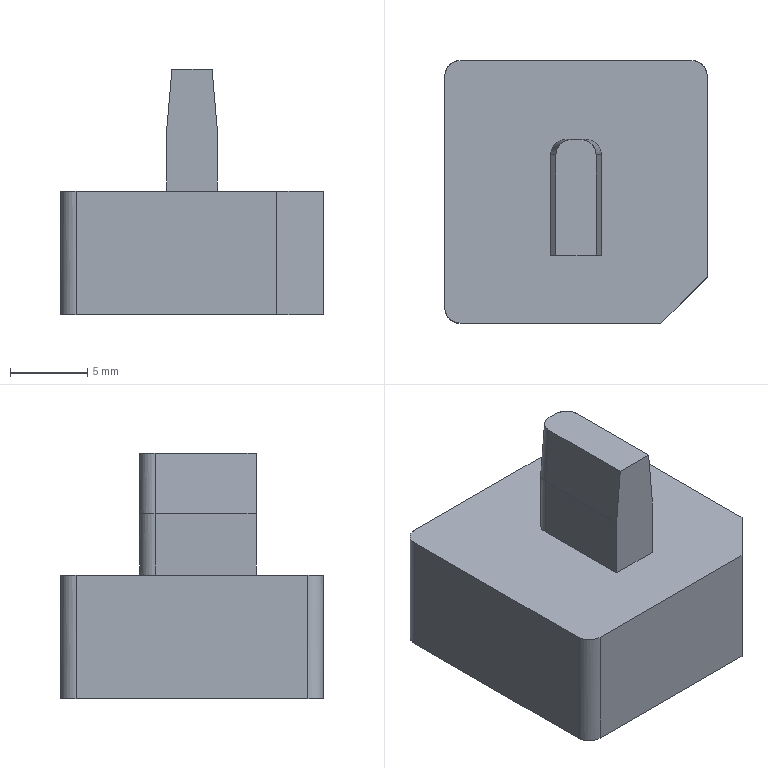NC program | PowerMill | posted with a generic post | part box 17 x 17 x 15.883 mm
Lines 3250 to 4049 of 22972:
N3347 M6
N3348 S18000 M03
N3349 G00 G90 X0.0 Y0.0
N3350 G43 Z10.804 H14
N3351
N3352 G05 P10000 R8
N3353 X2.8538 Y-6.1498
N3354 Z0.7597
N3355 G01 Z-0.4403 F1200.0
N3356 X2.8235 Y-6.0851 F2000.0
N3357 X2.7862 Y-6.0242
N3358 X2.7423 Y-5.9678
N3359 X2.6924 Y-5.9166
N3360 X2.6371 Y-5.8714
N3361 X2.5772 Y-5.8326
N3362 X2.5132 Y-5.8007
N3363 X2.4462 Y-5.7761
N3364 X2.3768 Y-5.7592
N3365 X2.3059 Y-5.7501
N3366 X2.2344 Y-5.749
N3367 X2.1633 Y-5.7558
N3368 X2.0934 Y-5.7705
N3369 X2.0256 Y-5.7929
N3370 X2.0213 Y-5.7946
N3371 X1.9047 Y-5.8415
N3372 X1.7934 Y-5.8786
N3373 X1.686 Y-5.9066
N3374 X1.5816 Y-5.9261
N3375 X1.4789 Y-5.9375
N3376 X1.3755 Y-5.9412
N3377 X0.4649 Y-5.9437
N3378 X-0.4456 Y-5.9451
N3379 X-1.2238 Y-5.9466
N3380 X-1.3612 Y-5.9432
N3381 X-1.4915 Y-5.9327
N3382 X-1.6155 Y-5.9151
N3383 X-1.7339 Y-5.8907
N3384 X-1.8472 Y-5.8595
N3385 X-1.9561 Y-5.8215
N3386 X-2.0624 Y-5.7761
N3387 X-2.1685 Y-5.7221
N3388 X-2.2712 Y-5.6609
N3389 X-2.3699 Y-5.5928
N3390 X-2.4639 Y-5.5183
N3391 X-2.5526 Y-5.4378
N3392 X-2.6354 Y-5.3519
N3393 X-2.7121 Y-5.2609
N3394 X-2.7835 Y-5.164
N3395 X-2.8481 Y-5.0626
N3396 X-2.9059 Y-4.9574
N3397 X-2.9564 Y-4.8488
N3398 X-2.9994 Y-4.7375
N3399 X-3.0346 Y-4.624
N3400 X-3.0621 Y-4.5089
N3401 X-3.0817 Y-4.3927
N3402 X-3.0934 Y-4.2758
N3403 X-3.0971 Y-4.1584
N3404 X-3.0972 Y0.4527
N3405 X-3.0979 Y2.3668
N3406 X-3.094 Y2.5191
N3407 X-3.0823 Y2.6701
N3408 X-3.0628 Y2.8197
N3409 X-3.0355 Y2.9674
N3410 X-3.0006 Y3.113
N3411 X-2.958 Y3.2562
N3412 X-2.9079 Y3.3967
N3413 X-2.8504 Y3.534
N3414 X-2.7856 Y3.6681
N3415 X-2.7137 Y3.7986
N3416 X-2.6348 Y3.9253
N3417 X-2.5491 Y4.0479
N3418 X-2.4574 Y4.1653
N3419 X-2.3593 Y4.2779
N3420 X-2.2552 Y4.3852
N3421 X-2.1456 Y4.4868
N3422 X-2.031 Y4.5821
N3423 X-1.9119 Y4.6707
N3424 X-1.7888 Y4.7525
N3425 X-1.6656 Y4.8253
N3426 X-1.5409 Y4.8911
N3427 X-1.4119 Y4.9512
N3428 X-1.2784 Y5.0051
N3429 X-1.1403 Y5.0524
N3430 X-1.0001 Y5.0922
N3431 X-0.8587 Y5.1248
N3432 X-0.7148 Y5.1513
N3433 X-0.5856 Y5.1687
N3434 X-0.4682 Y5.1776
N3435 X-0.3536 Y5.1796
N3436 X0.1899 Y5.1818
N3437 X0.3558 Y5.181
N3438 X0.5086 Y5.1736
N3439 X0.5739 Y5.168
N3440 X0.6389 Y5.1604
N3441 X0.7039 Y5.1518
N3442 X0.7686 Y5.1421
N3443 X0.8331 Y5.1304
N3444 X0.978 Y5.0983
N3445 X1.1212 Y5.0584
N3446 X1.2624 Y5.0108
N3447 X1.4012 Y4.9556
N3448 X1.5373 Y4.8929
N3449 X1.67 Y4.8229
N3450 X1.7991 Y4.7458
N3451 X1.9228 Y4.6627
N3452 X2.042 Y4.573
N3453 X2.1563 Y4.4771
N3454 X2.2653 Y4.3752
N3455 X2.3687 Y4.2676
N3456 X2.4661 Y4.1547
N3457 X2.5573 Y4.0368
N3458 X2.642 Y3.9142
N3459 X2.72 Y3.7872
N3460 X2.7911 Y3.6563
N3461 X2.8552 Y3.5214
N3462 X2.9122 Y3.3831
N3463 X2.9618 Y3.2416
N3464 X3.004 Y3.0973
N3465 X3.0385 Y2.9507
N3466 X3.0652 Y2.8023
N3467 X3.084 Y2.6525
N3468 X3.095 Y2.5017
N3469 X3.0981 Y2.3503
N3470 X3.0971 Y-2.801
N3471 Y-4.1623
N3472 X3.0931 Y-4.2787
N3473 X3.0812 Y-4.3949
N3474 X3.0613 Y-4.5107
N3475 X3.0335 Y-4.6258
N3476 X2.9978 Y-4.7395
N3477 X2.9544 Y-4.8513
N3478 X2.9033 Y-4.9605
N3479 X2.8449 Y-5.0667
N3480 X2.7808 Y-5.1671
N3481 X2.7102 Y-5.2631
N3482 X2.6333 Y-5.3543
N3483 X2.5503 Y-5.4402
N3484 X2.4617 Y-5.5205
N3485 X2.368 Y-5.5947
N3486 X2.2698 Y-5.6622
N3487 X2.1675 Y-5.7229
N3488 X2.0615 Y-5.7765
N3489 X2.0213 Y-5.7946
N3490 X1.915 Y-5.8366 Z-0.4405
N3491 X1.7985 Y-5.8747 Z-0.4407
N3492 X1.6832 Y-5.9045 Z-0.4409
N3493 X1.5738 Y-5.9254 Z-0.4411
N3494 X1.4717 Y-5.9377 Z-0.4412
N3495 X1.3752 Y-5.9423 Z-0.4414
N3496 X0.956 Y-5.9458 Z-0.442
N3497 X0.3745 Y-5.9446 Z-0.4429
N3498 X-0.3093 Y-5.9438 Z-0.444
N3499 X-1.3872 Y-5.9415 Z-0.4457
N3500 X-1.4857 Y-5.9372 Z-0.4458
N3501 X-1.5876 Y-5.9249 Z-0.446
N3502 X-1.6932 Y-5.9044 Z-0.4462
N3503 X-1.8027 Y-5.8751 Z-0.4463
N3504 X-1.9164 Y-5.8366 Z-0.4465
N3505 X-2.0345 Y-5.7885 Z-0.4467
N3506 X-2.1395 Y-5.7381 Z-0.4469
N3507 X-2.2415 Y-5.6803 Z-0.4471
N3508 X-2.3402 Y-5.6152 Z-0.4473
N3509 X-2.4349 Y-5.5431 Z-0.4475
N3510 X-2.5253 Y-5.4644 Z-0.4477
N3511 X-2.6102 Y-5.3799 Z-0.4478
N3512 X-2.6891 Y-5.2903 Z-0.448
N3513 X-2.762 Y-5.1956 Z-0.4482
N3514 X-2.8284 Y-5.0963 Z-0.4484
N3515 X-2.8881 Y-4.9929 Z-0.4486
N3516 X-2.9407 Y-4.8856 Z-0.4488
N3517 X-2.9861 Y-4.7752 Z-0.449
N3518 X-3.0239 Y-4.6621 Z-0.4491
N3519 X-3.054 Y-4.5471 Z-0.4493
N3520 X-3.0762 Y-4.4306 Z-0.4495
N3521 X-3.0905 Y-4.3133 Z-0.4497
N3522 X-3.0968 Y-4.1954 Z-0.4499
N3523 X-3.0972 Y-4.0773 Z-0.4501
N3524 X-3.0984 Y-0.148 Z-0.4562
N3525 X-3.0994 Y2.3669 Z-0.4601
N3526 X-3.0956 Y2.5199 Z-0.4603
N3527 X-3.0839 Y2.6713 Z-0.4606
N3528 X-3.0645 Y2.8207 Z-0.4608
N3529 X-3.0374 Y2.9681 Z-0.4611
N3530 X-3.0026 Y3.1132 Z-0.4613
N3531 X-2.9602 Y3.2559 Z-0.4615
N3532 X-2.9102 Y3.3958 Z-0.4617
N3533 X-2.8528 Y3.5328 Z-0.462
N3534 X-2.7881 Y3.6668 Z-0.4622
N3535 X-2.7161 Y3.7976 Z-0.4624
N3536 X-2.6369 Y3.9249 Z-0.4627
N3537 X-2.5523 Y4.0464 Z-0.4629
N3538 X-2.4609 Y4.1638 Z-0.4631
N3539 X-2.3634 Y4.276 Z-0.4634
N3540 X-2.26 Y4.3829 Z-0.4636
N3541 X-2.1509 Y4.4841 Z-0.4638
N3542 X-2.0364 Y4.5796 Z-0.4641
N3543 X-1.9167 Y4.6689 Z-0.4643
N3544 X-1.7922 Y4.7519 Z-0.4645
N3545 X-1.6633 Y4.8283 Z-0.4648
N3546 X-1.5303 Y4.8977 Z-0.465
N3547 X-1.3937 Y4.96 Z-0.4652
N3548 X-1.254 Y5.015 Z-0.4655
N3549 X-1.1116 Y5.0625 Z-0.4657
N3550 X-0.9668 Y5.1024 Z-0.4659
N3551 X-0.8401 Y5.1305 Z-0.4661
N3552 X-0.7087 Y5.1519 Z-0.4663
N3553 X-0.5649 Y5.1678 Z-0.4666
N3554 X-0.4029 Y5.1781 Z-0.4668
N3555 X-0.2102 Y5.1831 Z-0.4671
N3556 X0.0 Y5.184 Z-0.4675
N3557 X0.2448 Y5.1824 Z-0.4678
N3558 X0.4333 Y5.1762 Z-0.4681
N3559 X0.5951 Y5.1645 Z-0.4684
N3560 X0.7401 Y5.1472 Z-0.4686
N3561 X0.8714 Y5.1245 Z-0.4688
N3562 X1.0049 Y5.0934 Z-0.469
N3563 X1.1419 Y5.0534 Z-0.4693
N3564 X1.2827 Y5.0042 Z-0.4695
N3565 X1.4225 Y4.9473 Z-0.4697
N3566 X1.5586 Y4.8835 Z-0.47
N3567 X1.6908 Y4.8127 Z-0.4702
N3568 X1.8187 Y4.7351 Z-0.4704
N3569 X1.9421 Y4.651 Z-0.4707
N3570 X2.0607 Y4.5606 Z-0.4709
N3571 X2.174 Y4.464 Z-0.4711
N3572 X2.282 Y4.3616 Z-0.4714
N3573 X2.3842 Y4.2535 Z-0.4716
N3574 X2.4806 Y4.1401 Z-0.4718
N3575 X2.5709 Y4.0216 Z-0.472
N3576 X2.6548 Y3.8984 Z-0.4723
N3577 X2.732 Y3.771 Z-0.4725
N3578 X2.8022 Y3.6398 Z-0.4727
N3579 X2.8654 Y3.505 Z-0.473
N3580 X2.9213 Y3.367 Z-0.4732
N3581 X2.9698 Y3.2259 Z-0.4734
N3582 X3.0108 Y3.082 Z-0.4737
N3583 X3.0442 Y2.9357 Z-0.4739
N3584 X3.0699 Y2.7873 Z-0.4741
N3585 X3.0878 Y2.6371 Z-0.4744
N3586 X3.0978 Y2.4854 Z-0.4746
N3587 X3.1001 Y2.3327 Z-0.4749
N3588 X3.1006 Y-0.5346 Z-0.4793
N3589 X3.101 Y-3.0697 Z-0.4833
N3590 X3.1002 Y-4.1649 Z-0.485
N3591 X3.0961 Y-4.2821 Z-0.4852
N3592 X3.084 Y-4.3988 Z-0.4853
N3593 X3.064 Y-4.515 Z-0.4855
N3594 X3.0361 Y-4.63 Z-0.4857
N3595 X3.0005 Y-4.7435 Z-0.4859
N3596 X2.9571 Y-4.8548 Z-0.4861
N3597 X2.9062 Y-4.9634 Z-0.4863
N3598 X2.848 Y-5.0687 Z-0.4865
N3599 X2.7829 Y-5.1701 Z-0.4866
N3600 X2.7112 Y-5.267 Z-0.4868
N3601 X2.6344 Y-5.3575 Z-0.487
N3602 X2.5515 Y-5.4429 Z-0.4872
N3603 X2.463 Y-5.5227 Z-0.4874
N3604 X2.3692 Y-5.5965 Z-0.4876
N3605 X2.2705 Y-5.6641 Z-0.4878
N3606 X2.1674 Y-5.7249 Z-0.488
N3607 X2.0605 Y-5.7787 Z-0.4881
N3608 X2.0219 Y-5.796 Z-0.4882
N3609 X1.899 Y-5.8437 Z-0.4884
N3610 X1.7834 Y-5.8811 Z-0.4886
N3611 X1.6736 Y-5.909 Z-0.4888
N3612 X1.5684 Y-5.9282 Z-0.4889
N3613 X1.4674 Y-5.939 Z-0.4891
N3614 X1.3689 Y-5.9421 Z-0.4893
N3615 X0.4115 Y-5.9442 Z-0.4907
N3616 X-0.5216 Y-5.9455 Z-0.4922
N3617 X-1.1701 Y-5.9444 Z-0.4932
N3618 X-1.3875 Y-5.9425 Z-0.4935
N3619 X-1.4787 Y-5.9379 Z-0.4937
N3620 X-1.572 Y-5.9265 Z-0.4938
N3621 X-1.6751 Y-5.9072 Z-0.494
N3622 X-1.7875 Y-5.8791 Z-0.4942
N3623 X-1.9057 Y-5.8416 Z-0.4944
N3624 X-2.0173 Y-5.7983 Z-0.4946
N3625 X-2.1171 Y-5.7523 Z-0.4947
N3626 X-2.2043 Y-5.7052 Z-0.4949
N3627 X-2.2867 Y-5.6541 Z-0.495
N3628 X-2.3863 Y-5.584 Z-0.4952
N3629 X-2.48 Y-5.5085 Z-0.4954
N3630 X-2.5674 Y-5.428 Z-0.4956
N3631 X-2.6487 Y-5.3424 Z-0.4958
N3632 X-2.7253 Y-5.2504 Z-0.496
N3633 X-2.7957 Y-5.1535 Z-0.4962
N3634 X-2.8595 Y-5.0522 Z-0.4963
N3635 X-2.9163 Y-4.947 Z-0.4965
N3636 X-2.9659 Y-4.8383 Z-0.4967
N3637 X-3.0082 Y-4.7268 Z-0.4969
N3638 X-3.0427 Y-4.613 Z-0.4971
N3639 X-3.0694 Y-4.4975 Z-0.4973
N3640 X-3.0882 Y-4.3809 Z-0.4975
N3641 X-3.0991 Y-4.2637 Z-0.4976
N3642 X-3.1021 Y-4.1461 Z-0.4978
N3643 X-3.1029 Y1.1086 Z-0.506
N3644 X-3.1036 Y2.3669 Z-0.508
N3645 X-3.0998 Y2.5199 Z-0.5082
N3646 X-3.0881 Y2.6712 Z-0.5084
N3647 X-3.0687 Y2.8207 Z-0.5087
N3648 X-3.0416 Y2.968 Z-0.5089
N3649 X-3.0068 Y3.1131 Z-0.5091
N3650 X-2.9644 Y3.2557 Z-0.5094
N3651 X-2.9144 Y3.3957 Z-0.5096
N3652 X-2.857 Y3.5327 Z-0.5098
N3653 X-2.7923 Y3.6668 Z-0.5101
N3654 X-2.7202 Y3.7976 Z-0.5103
N3655 X-2.641 Y3.9251 Z-0.5105
N3656 X-2.5568 Y4.0461 Z-0.5108
N3657 X-2.4658 Y4.1629 Z-0.511
N3658 X-2.3688 Y4.2747 Z-0.5112
N3659 X-2.2657 Y4.3813 Z-0.5115
N3660 X-2.1567 Y4.4825 Z-0.5117
N3661 X-2.0422 Y4.578 Z-0.5119
N3662 X-1.9225 Y4.6674 Z-0.5122
N3663 X-1.7979 Y4.7506 Z-0.5124
N3664 X-1.6688 Y4.8271 Z-0.5126
N3665 X-1.5356 Y4.8968 Z-0.5129
N3666 X-1.3989 Y4.9593 Z-0.5131
N3667 X-1.2591 Y5.0144 Z-0.5133
N3668 X-1.1167 Y5.062 Z-0.5136
N3669 X-0.9722 Y5.1019 Z-0.5138
N3670 X-0.845 Y5.1302 Z-0.514
N3671 X-0.7136 Y5.1518 Z-0.5142
N3672 X-0.57 Y5.1677 Z-0.5144
N3673 X-0.4089 Y5.1779 Z-0.5147
N3674 X-0.2189 Y5.1828 Z-0.515
N3675 X-0.0002 Y5.1832 Z-0.5153
N3676 X0.253 Y5.1811 Z-0.5157
N3677 X0.4429 Y5.1748 Z-0.516
N3678 X0.6041 Y5.1632 Z-0.5163
N3679 X0.7477 Y5.1462 Z-0.5165
N3680 X0.8753 Y5.124 Z-0.5167
N3681 X1.0061 Y5.0934 Z-0.5169
N3682 X1.1429 Y5.0535 Z-0.5171
N3683 X1.2872 Y5.0033 Z-0.5174
N3684 X1.4203 Y4.9501 Z-0.5176
N3685 X1.5512 Y4.8896 Z-0.5178
N3686 X1.6805 Y4.821 Z-0.518
N3687 X1.8079 Y4.7446 Z-0.5183
N3688 X1.9321 Y4.6607 Z-0.5185
N3689 X2.0516 Y4.5706 Z-0.5187
N3690 X2.1661 Y4.4743 Z-0.519
N3691 X2.2751 Y4.372 Z-0.5192
N3692 X2.3786 Y4.2642 Z-0.5194
N3693 X2.476 Y4.151 Z-0.5197
N3694 X2.5671 Y4.0329 Z-0.5199
N3695 X2.6517 Y3.9102 Z-0.5201
N3696 X2.7295 Y3.7833 Z-0.5204
N3697 X2.8005 Y3.6524 Z-0.5206
N3698 X2.8643 Y3.518 Z-0.5208
N3699 X2.9209 Y3.3803 Z-0.521
N3700 X2.97 Y3.2403 Z-0.5213
N3701 X3.0116 Y3.098 Z-0.5215
N3702 X3.0455 Y2.9534 Z-0.5217
N3703 X3.0718 Y2.8064 Z-0.522
N3704 X3.0904 Y2.6571 Z-0.5222
N3705 X3.1012 Y2.5055 Z-0.5224
N3706 X3.1043 Y2.3515 Z-0.5227
N3707 X3.1048 Y-0.7272 Z-0.5275
N3708 X3.105 Y-3.5041 Z-0.5318
N3709 X3.1045 Y-4.1649 Z-0.5328
N3710 X3.1004 Y-4.2817 Z-0.533
N3711 X3.0884 Y-4.3981 Z-0.5332
N3712 X3.0684 Y-4.5142 Z-0.5334
N3713 X3.0405 Y-4.6293 Z-0.5336
N3714 X3.0047 Y-4.7429 Z-0.5338
N3715 X2.9612 Y-4.8545 Z-0.5339
N3716 X2.9102 Y-4.9635 Z-0.5341
N3717 X2.8519 Y-5.0692 Z-0.5343
N3718 X2.7876 Y-5.1695 Z-0.5345
N3719 X2.7167 Y-5.2655 Z-0.5347
N3720 X2.6395 Y-5.3566 Z-0.5349
N3721 X2.5564 Y-5.4423 Z-0.5351
N3722 X2.4677 Y-5.5223 Z-0.5352
N3723 X2.3738 Y-5.5962 Z-0.5354
N3724 X2.2752 Y-5.6637 Z-0.5356
N3725 X2.1724 Y-5.7244 Z-0.5358
N3726 X2.0658 Y-5.7781 Z-0.536
N3727 X2.0224 Y-5.7974 Z-0.5361
N3728 X1.902 Y-5.8438 Z-0.5363
N3729 X1.7859 Y-5.8808 Z-0.5365
N3730 X1.6736 Y-5.9087 Z-0.5366
N3731 X1.5648 Y-5.928 Z-0.5368
N3732 X1.4593 Y-5.9392 Z-0.537
N3733 X1.3555 Y-5.9427 Z-0.5371
N3734 X0.9251 Y-5.9459 Z-0.5378
N3735 X0.3142 Y-5.9444 Z-0.5388
N3736 X-0.38 Y-5.9437 Z-0.5398
N3737 X-1.3872 Y-5.9417 Z-0.5414
N3738 X-1.4904 Y-5.9374 Z-0.5416
N3739 X-1.5956 Y-5.9251 Z-0.5417
N3740 X-1.7028 Y-5.9047 Z-0.5419
N3741 X-1.8119 Y-5.8759 Z-0.5421
N3742 X-1.9226 Y-5.8385 Z-0.5423
N3743 X-2.0346 Y-5.7924 Z-0.5424
N3744 X-2.1474 Y-5.7375 Z-0.5426
N3745 X-2.2476 Y-5.6812 Z-0.5428
N3746 X-2.3443 Y-5.6181 Z-0.543
N3747 X-2.4379 Y-5.5476 Z-0.5432
N3748 X-2.5278 Y-5.4699 Z-0.5434
N3749 X-2.6108 Y-5.3882 Z-0.5435
N3750 X-2.6903 Y-5.299 Z-0.5437
N3751 X-2.7637 Y-5.2048 Z-0.5439
N3752 X-2.8308 Y-5.106 Z-0.5441
N3753 X-2.8911 Y-5.0029 Z-0.5443
N3754 X-2.9444 Y-4.896 Z-0.5445
N3755 X-2.9905 Y-4.7858 Z-0.5447
N3756 X-3.029 Y-4.673 Z-0.5448
N3757 X-3.0598 Y-4.5581 Z-0.545
N3758 X-3.0828 Y-4.4417 Z-0.5452
N3759 X-3.0978 Y-4.3244 Z-0.5454
N3760 X-3.1049 Y-4.2066 Z-0.5456
N3761 X-3.1056 Y-4.0886 Z-0.5458
N3762 X-3.1068 Y-0.1506 Z-0.5519
N3763 X-3.1078 Y2.3669 Z-0.5558
N3764 X-3.104 Y2.5199 Z-0.5561
N3765 X-3.0924 Y2.6713 Z-0.5563
N3766 X-3.0729 Y2.8208 Z-0.5565
N3767 X-3.0458 Y2.9682 Z-0.5568
N3768 X-3.011 Y3.1134 Z-0.557
N3769 X-2.9685 Y3.256 Z-0.5572
N3770 X-2.9186 Y3.396 Z-0.5575
N3771 X-2.8612 Y3.5331 Z-0.5577
N3772 X-2.7964 Y3.6672 Z-0.5579
N3773 X-2.7244 Y3.7981 Z-0.5582
N3774 X-2.6452 Y3.9255 Z-0.5584
N3775 X-2.5612 Y4.0462 Z-0.5586
N3776 X-2.4706 Y4.1626 Z-0.5588
N3777 X-2.3736 Y4.2742 Z-0.5591
N3778 X-2.2703 Y4.3809 Z-0.5593
N3779 X-2.1611 Y4.4823 Z-0.5595
N3780 X-2.0462 Y4.578 Z-0.5598
N3781 X-1.9259 Y4.6679 Z-0.56
N3782 X-1.8006 Y4.7515 Z-0.5602
N3783 X-1.6732 Y4.8272 Z-0.5605
N3784 X-1.5417 Y4.8961 Z-0.5607
N3785 X-1.4067 Y4.9579 Z-0.5609
N3786 X-1.2683 Y5.0125 Z-0.5612
N3787 X-1.1267 Y5.0597 Z-0.5614
N3788 X-0.9825 Y5.0993 Z-0.5616
N3789 X-0.8359 Y5.1317 Z-0.5619
N3790 X-0.7097 Y5.1544 Z-0.5621
N3791 X-0.6028 Y5.1674 Z-0.5622
N3792 X-0.5001 Y5.1738 Z-0.5624
N3793 X-0.298 Y5.1803 Z-0.5627
N3794 X-0.0349 Y5.1821 Z-0.5631
N3795 X0.229 Y5.1812 Z-0.5635
N3796 X0.4226 Y5.176 Z-0.5638
N3797 X0.5862 Y5.1655 Z-0.5641
N3798 X0.7319 Y5.1495 Z-0.5643
N3799 X0.8616 Y5.1283 Z-0.5645
N3800 X0.993 Y5.0989 Z-0.5647
N3801 X1.1283 Y5.0606 Z-0.5649
N3802 X1.2677 Y5.0131 Z-0.5652
N3803 X1.4107 Y4.956 Z-0.5654
N3804 X1.5485 Y4.8927 Z-0.5657
N3805 X1.6806 Y4.8234 Z-0.5659
N3806 X1.8071 Y4.7482 Z-0.5661
N3807 X1.9285 Y4.667 Z-0.5663
N3808 X2.048 Y4.5774 Z-0.5666
N3809 X2.1626 Y4.4815 Z-0.5668
N3810 X2.272 Y4.3797 Z-0.567
N3811 X2.3757 Y4.2721 Z-0.5673
N3812 X2.4736 Y4.1591 Z-0.5675
N3813 X2.5652 Y4.0412 Z-0.5677
N3814 X2.6503 Y3.9187 Z-0.568
N3815 X2.7287 Y3.7918 Z-0.5682
N3816 X2.8002 Y3.6609 Z-0.5684
N3817 X2.8644 Y3.5266 Z-0.5687
N3818 X2.9217 Y3.3888 Z-0.5689
N3819 X2.9713 Y3.2489 Z-0.5691
N3820 X3.0134 Y3.1068 Z-0.5694
N3821 X3.0478 Y2.9625 Z-0.5696
N3822 X3.0745 Y2.816 Z-0.5698
N3823 X3.0936 Y2.6671 Z-0.5701
N3824 X3.1049 Y2.5159 Z-0.5703
N3825 X3.1085 Y2.3668 Z-0.5705
N3826 X3.109 Y-0.7272 Z-0.5753
N3827 X3.1092 Y-3.3491 Z-0.5794
N3828 X3.1082 Y-4.165 Z-0.5807
N3829 X3.104 Y-4.2828 Z-0.5809
N3830 X3.0919 Y-4.4 Z-0.5811
N3831 X3.0718 Y-4.5165 Z-0.5812
N3832 X3.0439 Y-4.6318 Z-0.5814
N3833 X3.0081 Y-4.7454 Z-0.5816
N3834 X2.9647 Y-4.8568 Z-0.5818
N3835 X2.9138 Y-4.9653 Z-0.582
N3836 X2.8557 Y-5.0704 Z-0.5822
N3837 X2.7918 Y-5.17 Z-0.5824
N3838 X2.7211 Y-5.2653 Z-0.5825
N3839 X2.6438 Y-5.3564 Z-0.5827
N3840 X2.5602 Y-5.4424 Z-0.5829
N3841 X2.4709 Y-5.5229 Z-0.5831
N3842 X2.3768 Y-5.597 Z-0.5833
N3843 X2.2785 Y-5.6643 Z-0.5835
N3844 X2.1766 Y-5.7245 Z-0.5837
N3845 X2.072 Y-5.7771 Z-0.5838
N3846 X2.0229 Y-5.7988 Z-0.5839
N3847 X1.9036 Y-5.8448 Z-0.5841
N3848 X1.7878 Y-5.8814 Z-0.5843
N3849 X1.6754 Y-5.9091 Z-0.5845
N3850 X1.5662 Y-5.9284 Z-0.5847
N3851 X1.4599 Y-5.9394 Z-0.5848
N3852 X1.3553 Y-5.9429 Z-0.585
N3853 X0.9104 Y-5.9458 Z-0.5857
N3854 X0.2674 Y-5.9444 Z-0.5867
N3855 X-0.4484 Y-5.9437 Z-0.5878
N3856 X-1.3872 Y-5.9419 Z-0.5893
N3857 X-1.4911 Y-5.9376 Z-0.5894
N3858 X-1.5969 Y-5.9254 Z-0.5896
N3859 X-1.7046 Y-5.905 Z-0.5898
N3860 X-1.8142 Y-5.8762 Z-0.5899
N3861 X-1.9252 Y-5.839 Z-0.5901
N3862 X-2.0374 Y-5.793 Z-0.5903
N3863 X-2.15 Y-5.7384 Z-0.5905
N3864 X-2.2506 Y-5.682 Z-0.5907
N3865 X-2.3477 Y-5.6187 Z-0.5909
N3866 X-2.4414 Y-5.5481 Z-0.591
N3867 X-2.5314 Y-5.4704 Z-0.5912
N3868 X-2.6158 Y-5.3873 Z-0.5914
N3869 X-2.6955 Y-5.2978 Z-0.5916
N3870 X-2.7691 Y-5.2033 Z-0.5918
N3871 X-2.8362 Y-5.1043 Z-0.592
N3872 X-2.8966 Y-5.001 Z-0.5922
N3873 X-2.95 Y-4.8941 Z-0.5923
N3874 X-2.996 Y-4.7839 Z-0.5925
N3875 X-3.0345 Y-4.6712 Z-0.5927
N3876 X-3.0652 Y-4.5565 Z-0.5929
N3877 X-3.088 Y-4.4404 Z-0.5931
N3878 X-3.103 Y-4.3235 Z-0.5933
N3879 X-3.1099 Y-4.206 Z-0.5934
N3880 X-3.1105 Y-4.0883 Z-0.5936
N3881 X-3.1113 Y2.0274 Z-0.6031
N3882 X-3.1114 Y2.3669 Z-0.6037
N3883 X-3.1076 Y2.5219 Z-0.6039
N3884 X-3.096 Y2.6741 Z-0.6042
N3885 X-3.0767 Y2.8233 Z-0.6044
N3886 X-3.0501 Y2.969 Z-0.6046
N3887 X-3.0161 Y3.111 Z-0.6048
N3888 X-2.9748 Y3.2502 Z-0.6051
N3889 X-2.9247 Y3.3912 Z-0.6053
N3890 X-2.8671 Y3.5293 Z-0.6055
N3891 X-2.8022 Y3.6641 Z-0.6058
N3892 X-2.7301 Y3.7954 Z-0.606
N3893 X-2.6512 Y3.9226 Z-0.6062
N3894 X-2.5656 Y4.0454 Z-0.6065
N3895 X-2.4736 Y4.1634 Z-0.6067
N3896 X-2.3754 Y4.2764 Z-0.6069
N3897 X-2.2732 Y4.382 Z-0.6072
N3898 X-2.1651 Y4.4824 Z-0.6074
N3899 X-2.051 Y4.5775 Z-0.6076
N3900 X-1.9312 Y4.6668 Z-0.6079
N3901 X-1.8063 Y4.7501 Z-0.6081
N3902 X-1.6766 Y4.827 Z-0.6083
N3903 X-1.5428 Y4.897 Z-0.6086
N3904 X-1.4054 Y4.9599 Z-0.6088
N3905 X-1.2651 Y5.0154 Z-0.609
N3906 X-1.1225 Y5.0632 Z-0.6093
N3907 X-0.9783 Y5.1031 Z-0.6095
N3908 X-0.8536 Y5.131 Z-0.6097
N3909 X-0.7251 Y5.1522 Z-0.6099
N3910 X-0.5843 Y5.1677 Z-0.6101
N3911 X-0.4258 Y5.1777 Z-0.6104
N3912 X-0.2374 Y5.1823 Z-0.6107
N3913 X0.0 Y5.1828 Z-0.611
N3914 X0.2549 Y5.1811 Z-0.6114
N3915 X0.4462 Y5.1751 Z-0.6117
N3916 X0.6089 Y5.1638 Z-0.612
N3917 X0.7542 Y5.147 Z-0.6122
N3918 X0.8791 Y5.1257 Z-0.6124
N3919 X1.008 Y5.096 Z-0.6126
N3920 X1.1432 Y5.0568 Z-0.6128
N3921 X1.2843 Y5.0079 Z-0.6131
N3922 X1.4297 Y4.9494 Z-0.6133
N3923 X1.5453 Y4.8967 Z-0.6135
N3924 X1.6666 Y4.8341 Z-0.6137
N3925 X1.7885 Y4.7624 Z-0.6139
N3926 X1.9026 Y4.6873 Z-0.6141
N3927 X2.0132 Y4.6072 Z-0.6144
N3928 X2.1293 Y4.5138 Z-0.6146
N3929 X2.2402 Y4.4142 Z-0.6148
N3930 X2.3456 Y4.3089 Z-0.6151
N3931 X2.4453 Y4.1981 Z-0.6153
N3932 X2.539 Y4.082 Z-0.6155
N3933 X2.6264 Y3.9609 Z-0.6158
N3934 X2.7072 Y3.8353 Z-0.616
N3935 X2.7813 Y3.7055 Z-0.6162
N3936 X2.8482 Y3.5719 Z-0.6164
N3937 X2.908 Y3.4351 Z-0.6167
N3938 X2.9603 Y3.2953 Z-0.6169
N3939 X3.0051 Y3.1529 Z-0.6171
N3940 X3.0406 Y3.0158 Z-0.6174
N3941 X3.0692 Y2.8771 Z-0.6176
N3942 X3.0908 Y2.7349 Z-0.6178
N3943 X3.1052 Y2.5881 Z-0.618
N3944 X3.112 Y2.4415 Z-0.6183
N3945 X3.1128 Y2.2941 Z-0.6185
N3946 X3.1131 Y-0.7272 Z-0.6232
N3947 X3.1137 Y-3.8555 Z-0.6281
N3948 X3.1135 Y-4.165 Z-0.6285
N3949 X3.1095 Y-4.282 Z-0.6287
N3950 X3.0975 Y-4.3985 Z-0.6289
N3951 X3.0776 Y-4.5144 Z-0.6291
N3952 X3.0497 Y-4.6293 Z-0.6293
N3953 X3.0141 Y-4.7426 Z-0.6295
N3954 X2.9707 Y-4.8538 Z-0.6297
N3955 X2.9198 Y-4.9624 Z-0.6298
N3956 X2.8616 Y-5.0678 Z-0.63
N3957 X2.7964 Y-5.1694 Z-0.6302
N3958 X2.7265 Y-5.2639 Z-0.6304
N3959 X2.65 Y-5.3542 Z-0.6306
N3960 X2.5667 Y-5.4402 Z-0.6308
N3961 X2.4774 Y-5.5209 Z-0.631
N3962 X2.3831 Y-5.5954 Z-0.6311
N3963 X2.2849 Y-5.6629 Z-0.6313
N3964 X2.1838 Y-5.7229 Z-0.6315
N3965 X2.0805 Y-5.7751 Z-0.6317
N3966 X2.0235 Y-5.8002 Z-0.6318
N3967 X1.904 Y-5.8459 Z-0.632
N3968 X1.7883 Y-5.8824 Z-0.6322
N3969 X1.6761 Y-5.9099 Z-0.6324
N3970 X1.5672 Y-5.9289 Z-0.6325
N3971 X1.4613 Y-5.9397 Z-0.6327
N3972 X1.3571 Y-5.943 Z-0.6329
N3973 X0.8605 Y-5.9452 Z-0.6336
N3974 X0.1748 Y-5.944 Z-0.6347
N3975 X-1.3874 Y-5.9437 Z-0.6371
N3976 X-1.4522 Y-5.9408 Z-0.6372
N3977 X-1.5167 Y-5.9344 Z-0.6373
N3978 X-1.6053 Y-5.9219 Z-0.6375
N3979 X-1.6692 Y-5.9106 Z-0.6376
N3980 X-1.7326 Y-5.8967 Z-0.6377
N3981 X-1.8499 Y-5.8641 Z-0.6379
N3982 X-1.9648 Y-5.824 Z-0.638
N3983 X-2.0773 Y-5.7763 Z-0.6382
N3984 X-2.1877 Y-5.7209 Z-0.6384
N3985 X-2.2855 Y-5.6635 Z-0.6386
N3986 X-2.3804 Y-5.5987 Z-0.6388
N3987 X-2.4724 Y-5.5263 Z-0.639
N3988 X-2.5612 Y-5.4464 Z-0.6391
N3989 X-2.6449 Y-5.3606 Z-0.6393
N3990 X-2.7225 Y-5.2698 Z-0.6395
N3991 X-2.794 Y-5.1741 Z-0.6397
N3992 X-2.8589 Y-5.0739 Z-0.6399
N3993 X-2.917 Y-4.9695 Z-0.6401
N3994 X-2.9681 Y-4.8616 Z-0.6403
N3995 X-3.0118 Y-4.7505 Z-0.6404
N3996 X-3.0479 Y-4.637 Z-0.6406
N3997 X-3.0763 Y-4.5215 Z-0.6408
N3998 X-3.0967 Y-4.4048 Z-0.641
N3999 X-3.1093 Y-4.2873 Z-0.6412
N4000 X-3.1139 Y-4.1694 Z-0.6414
N4001 X-3.114 Y-4.0513 Z-0.6416
N4002 X-3.1151 Y-0.1566 Z-0.6476
N4003 X-3.1162 Y2.3669 Z-0.6515
N4004 X-3.1124 Y2.5196 Z-0.6518
N4005 X-3.1007 Y2.671 Z-0.652
N4006 X-3.0812 Y2.8207 Z-0.6522
N4007 X-3.0539 Y2.9685 Z-0.6525
N4008 X-3.0189 Y3.1141 Z-0.6527
N4009 X-2.9762 Y3.2572 Z-0.6529
N4010 X-2.9261 Y3.3976 Z-0.6532
N4011 X-2.8686 Y3.5351 Z-0.6534
N4012 X-2.8038 Y3.6694 Z-0.6536
N4013 X-2.7318 Y3.8002 Z-0.6539
N4014 X-2.6572 Y3.9206 Z-0.6541
N4015 X-2.576 Y4.0372 Z-0.6543
N4016 X-2.4848 Y4.1546 Z-0.6545
N4017 X-2.3853 Y4.2697 Z-0.6548
N4018 X-2.2827 Y4.3767 Z-0.655
N4019 X-2.1794 Y4.4738 Z-0.6552
N4020 X-2.0712 Y4.5652 Z-0.6554
N4021 X-1.9535 Y4.6544 Z-0.6557
N4022 X-1.83 Y4.738 Z-0.6559
N4023 X-1.7011 Y4.8156 Z-0.6561
N4024 X-1.5675 Y4.8867 Z-0.6564
N4025 X-1.43 Y4.9509 Z-0.6566
N4026 X-1.2894 Y5.0077 Z-0.6569
N4027 X-1.1468 Y5.0567 Z-0.6571
N4028 X-1.0029 Y5.0979 Z-0.6573
N4029 X-0.8793 Y5.1266 Z-0.6575
N4030 X-0.7538 Y5.1487 Z-0.6577
N4031 X-0.6167 Y5.1651 Z-0.6579
N4032 X-0.4631 Y5.1759 Z-0.6582
N4033 X-0.2825 Y5.1813 Z-0.6584
N4034 X-0.0413 Y5.1821 Z-0.6588
N4035 X0.0572 Y5.182 Z-0.659
N4036 X0.1556 Y5.1819 Z-0.6591
N4037 X0.2541 Y5.1816 Z-0.6593
N4038 X0.3525 Y5.181 Z-0.6594
N4039 X0.4509 Y5.1786 Z-0.6596
N4040 X0.582 Y5.1689 Z-0.6598
N4041 X0.7317 Y5.1504 Z-0.66
N4042 X0.8571 Y5.1302 Z-0.6602
N4043 X0.9855 Y5.1022 Z-0.6604
N4044 X1.1212 Y5.0646 Z-0.6606
N4045 X1.2638 Y5.0172 Z-0.6609
N4046 X1.4049 Y4.9622 Z-0.6611
N4047 X1.5416 Y4.9004 Z-0.6614
N4048 X1.6736 Y4.832 Z-0.6616
N4049 X1.8009 Y4.7572 Z-0.6618
N4050 X1.9253 Y4.6749 Z-0.662
N4051 X2.0452 Y4.5861 Z-0.6623
N4052 X2.1601 Y4.4909 Z-0.6625
N4053 X2.2699 Y4.3898 Z-0.6627
N4054 X2.3742 Y4.2829 Z-0.663
N4055 X2.4726 Y4.1705 Z-0.6632
N4056 X2.565 Y4.053 Z-0.6634
N4057 X2.6509 Y3.9308 Z-0.6637
N4058 X2.7301 Y3.8041 Z-0.6639
N4059 X2.8023 Y3.6736 Z-0.6641
N4060 X2.8675 Y3.5394 Z-0.6644
N4061 X2.9254 Y3.402 Z-0.6646
N4062 X2.9759 Y3.2616 Z-0.6648
N4063 X3.0188 Y3.1188 Z-0.6651
N4064 X3.0529 Y2.9796 Z-0.6653
N4065 X3.08 Y2.8381 Z-0.6655
N4066 X3.0998 Y2.6929 Z-0.6657
N4067 X3.1122 Y2.5443 Z-0.666
N4068 X3.117 Y2.3947 Z-0.6662
N4069 X3.1171 Y2.2434 Z-0.6664
N4070 X3.1177 Y-3.8127 Z-0.6759
N4071 Y-4.165 Z-0.6764
N4072 X3.1137 Y-4.2818 Z-0.6766
N4073 X3.1018 Y-4.3981 Z-0.6768
N4074 X3.082 Y-4.5138 Z-0.677
N4075 X3.0542 Y-4.6286 Z-0.6771
N4076 X3.0186 Y-4.7419 Z-0.6773
N4077 X2.9753 Y-4.8531 Z-0.6775
N4078 X2.9244 Y-4.9617 Z-0.6777
N4079 X2.8662 Y-5.0672 Z-0.6779
N4080 X2.8009 Y-5.1689 Z-0.6781
N4081 X2.7317 Y-5.2627 Z-0.6782
N4082 X2.6557 Y-5.3526 Z-0.6784
N4083 X2.5726 Y-5.4386 Z-0.6786
N4084 X2.4832 Y-5.5195 Z-0.6788
N4085 X2.3889 Y-5.5942 Z-0.679
N4086 X2.2909 Y-5.6618 Z-0.6792
N4087 X2.1903 Y-5.7217 Z-0.6794
N4088 X2.0881 Y-5.7735 Z-0.6795
N4089 X2.024 Y-5.8016 Z-0.6796
N4090 X1.9141 Y-5.8454 Z-0.6798
N4091 X1.8023 Y-5.8817 Z-0.68
N4092 X1.6914 Y-5.9097 Z-0.6802
N4093 X1.5832 Y-5.9293 Z-0.6804
N4094 X1.4791 Y-5.9405 Z-0.6805
N4095 X1.3793 Y-5.9439 Z-0.6807
N4096 X0.1749 Y-5.9444 Z-0.6825
N4097 X-0.464 Y-5.947 Z-0.6835
N4098 X-1.0031 Y-5.9478 Z-0.6844
N4099 X-1.3874 Y-5.9439 Z-0.685
N4100 X-1.4968 Y-5.938 Z-0.6851
N4101 X-1.6073 Y-5.9242 Z-0.6853
N4102 X-1.7191 Y-5.9022 Z-0.6855
N4103 X-1.8317 Y-5.8721 Z-0.6857
N4104 X-1.9448 Y-5.8336 Z-0.6859
N4105 X-2.0579 Y-5.7867 Z-0.6861
N4106 X-2.1706 Y-5.7316 Z-0.6862
N4107 X-2.2706 Y-5.6746 Z-0.6864
N4108 X-2.3673 Y-5.6106 Z-0.6866
N4109 X-2.4605 Y-5.5393 Z-0.6868
N4110 X-2.5499 Y-5.461 Z-0.687
N4111 X-2.6346 Y-5.3762 Z-0.6872
N4112 X-2.7133 Y-5.2864 Z-0.6873
N4113 X-2.7859 Y-5.1915 Z-0.6875
N4114 X-2.852 Y-5.092 Z-0.6877
N4115 X-2.9114 Y-4.9884 Z-0.6879
N4116 X-2.9637 Y-4.881 Z-0.6881
N4117 X-3.0088 Y-4.7705 Z-0.6883
N4118 X-3.0462 Y-4.6573 Z-0.6885
N4119 X-3.076 Y-4.5422 Z-0.6886
N4120 X-3.0979 Y-4.4257 Z-0.6888
N4121 X-3.1118 Y-4.3083 Z-0.689
N4122 X-3.1178 Y-4.1904 Z-0.6892
N4123 X-3.1182 Y-4.0723 Z-0.6894
N4124 X-3.1193 Y-0.1801 Z-0.6954
N4125 X-3.1204 Y2.3669 Z-0.6994
N4126 X-3.1166 Y2.5196 Z-0.6996
N4127 X-3.1049 Y2.671 Z-0.6999
N4128 X-3.0854 Y2.8207 Z-0.7001
N4129 X-3.0581 Y2.9685 Z-0.7003
N4130 X-3.0231 Y3.114 Z-0.7006
N4131 X-2.9805 Y3.2571 Z-0.7008
N4132 X-2.9304 Y3.3975 Z-0.701
N4133 X-2.8729 Y3.5349 Z-0.7013
N4134 X-2.8081 Y3.6691 Z-0.7015
N4135 X-2.7361 Y3.7999 Z-0.7017
N4136 X-2.6594 Y3.9235 Z-0.7019
N4137 X-2.5755 Y4.0437 Z-0.7022
N4138 X-2.4841 Y4.1607 Z-0.7024
N4139 X-2.3857 Y4.2738 Z-0.7026
N4140 X-2.2808 Y4.3822 Z-0.7029
N4141 X-2.1701 Y4.485 Z-0.7031
N4142 X-2.0547 Y4.5814 Z-0.7033
N4143 X-1.9355 Y4.6708 Z-0.7036
N4144 X-1.8206 Y4.7477 Z-0.7038
N4145 X-1.7 Y4.8194 Z-0.704
N4146 X-1.5699 Y4.8875 Z-0.7042